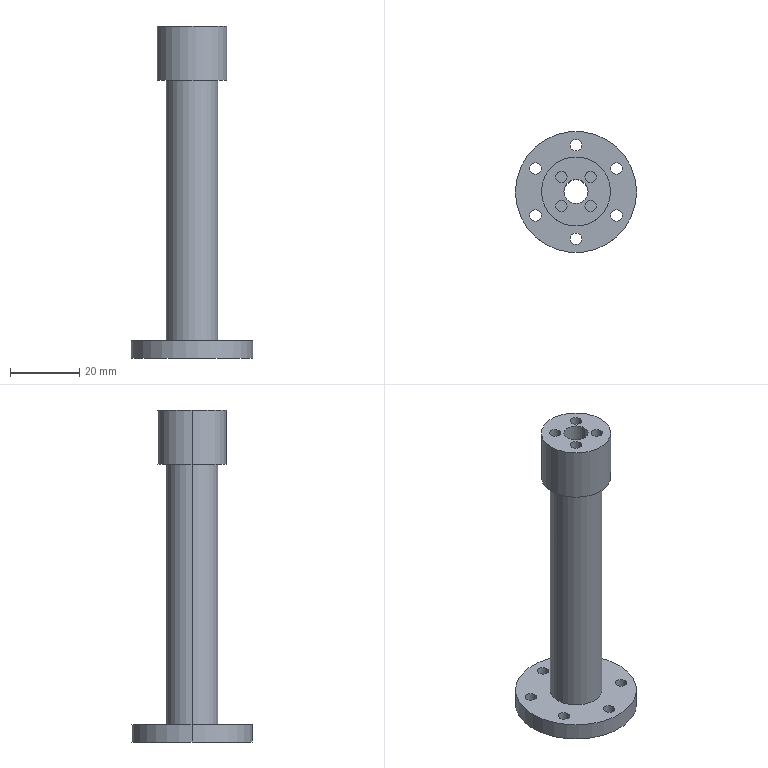Part | SolidWorks | features ICE 5, Extrusion 1 | 1 solid | 36 faces | box 35 x 35 x 95.91 mm | volume 18807 mm3 | cylinder 28 | plane 8 | commonest cylinder face diameters 3.3 x20 7 x2 15 x2 20 x2 35 x2
STEP:
#1=CARTESIAN_POINT('',(2.593,4.243,87.91));
#2=VERTEX_POINT('',#1);
#3=CARTESIAN_POINT('',(5.893,4.243,87.91));
#4=VERTEX_POINT('',#3);
#5=CARTESIAN_POINT('',(4.243,4.243,87.91));
#6=DIRECTION('',(0.,0.,1.));
#7=DIRECTION('',(1.,0.,0.));
#8=AXIS2_PLACEMENT_3D('',#5,#6,#7);
#9=CIRCLE('',#8,1.65);
#10=EDGE_CURVE('',#2,#4,#9,.T.);
#11=ORIENTED_EDGE('',*,*,#10,.F.);
#12=CARTESIAN_POINT('',(2.593,4.243,95.91));
#13=VERTEX_POINT('',#12);
#14=CARTESIAN_POINT('',(2.593,4.243,87.91));
#15=DIRECTION('',(0.,0.,1.));
#16=VECTOR('',#15,1000.);
#17=LINE('',#14,#16);
#18=EDGE_CURVE('',#2,#13,#17,.T.);
#19=ORIENTED_EDGE('',*,*,#18,.T.);
#20=CARTESIAN_POINT('',(5.893,4.243,95.91));
#21=VERTEX_POINT('',#20);
#22=CARTESIAN_POINT('',(4.243,4.243,95.91));
#23=DIRECTION('',(0.,0.,1.));
#24=DIRECTION('',(1.,0.,0.));
#25=AXIS2_PLACEMENT_3D('',#22,#23,#24);
#26=CIRCLE('',#25,1.65);
#27=EDGE_CURVE('',#13,#21,#26,.T.);
#28=ORIENTED_EDGE('',*,*,#27,.T.);
#29=CARTESIAN_POINT('',(5.893,4.243,87.91));
#30=DIRECTION('',(0.,0.,1.));
#31=VECTOR('',#30,1000.);
#32=LINE('',#29,#31);
#33=EDGE_CURVE('',#4,#21,#32,.T.);
#34=ORIENTED_EDGE('',*,*,#33,.F.);
#35=EDGE_LOOP('',(#11,#19,#28,#34));
#36=FACE_OUTER_BOUND('',#35,.T.);
#37=CARTESIAN_POINT('',(4.243,4.243,87.91));
#38=DIRECTION('',(0.,0.,1.));
#39=DIRECTION('',(1.,0.,0.));
#40=AXIS2_PLACEMENT_3D('',#37,#38,#39);
#41=CYLINDRICAL_SURFACE('',#40,1.65);
#42=ADVANCED_FACE('',(#36),#41,.F.);
#43=CARTESIAN_POINT('',(2.593,-4.243,87.91));
#44=VERTEX_POINT('',#43);
#45=CARTESIAN_POINT('',(5.893,-4.243,87.91));
#46=VERTEX_POINT('',#45);
#47=CARTESIAN_POINT('',(4.243,-4.243,87.91));
#48=DIRECTION('',(0.,0.,1.));
#49=DIRECTION('',(1.,0.,0.));
#50=AXIS2_PLACEMENT_3D('',#47,#48,#49);
#51=CIRCLE('',#50,1.65);
#52=EDGE_CURVE('',#44,#46,#51,.T.);
#53=ORIENTED_EDGE('',*,*,#52,.F.);
#54=CARTESIAN_POINT('',(2.593,-4.243,95.91));
#55=VERTEX_POINT('',#54);
#56=CARTESIAN_POINT('',(2.593,-4.243,87.91));
#57=DIRECTION('',(0.,0.,1.));
#58=VECTOR('',#57,1000.);
#59=LINE('',#56,#58);
#60=EDGE_CURVE('',#44,#55,#59,.T.);
#61=ORIENTED_EDGE('',*,*,#60,.T.);
#62=CARTESIAN_POINT('',(5.893,-4.243,95.91));
#63=VERTEX_POINT('',#62);
#64=CARTESIAN_POINT('',(4.243,-4.243,95.91));
#65=DIRECTION('',(0.,0.,1.));
#66=DIRECTION('',(1.,0.,0.));
#67=AXIS2_PLACEMENT_3D('',#64,#65,#66);
#68=CIRCLE('',#67,1.65);
#69=EDGE_CURVE('',#55,#63,#68,.T.);
#70=ORIENTED_EDGE('',*,*,#69,.T.);
#71=CARTESIAN_POINT('',(5.893,-4.243,87.91));
#72=DIRECTION('',(0.,0.,1.));
#73=VECTOR('',#72,1000.);
#74=LINE('',#71,#73);
#75=EDGE_CURVE('',#46,#63,#74,.T.);
#76=ORIENTED_EDGE('',*,*,#75,.F.);
#77=EDGE_LOOP('',(#53,#61,#70,#76));
#78=FACE_OUTER_BOUND('',#77,.T.);
#79=CARTESIAN_POINT('',(4.243,-4.243,87.91));
#80=DIRECTION('',(0.,0.,1.));
#81=DIRECTION('',(1.,0.,0.));
#82=AXIS2_PLACEMENT_3D('',#79,#80,#81);
#83=CYLINDRICAL_SURFACE('',#82,1.65);
#84=ADVANCED_FACE('',(#78),#83,.F.);
#85=CARTESIAN_POINT('',(-5.893,-4.243,87.91));
#86=VERTEX_POINT('',#85);
#87=CARTESIAN_POINT('',(-2.593,-4.243,87.91));
#88=VERTEX_POINT('',#87);
#89=CARTESIAN_POINT('',(-4.243,-4.243,87.91));
#90=DIRECTION('',(0.,0.,1.));
#91=DIRECTION('',(1.,0.,0.));
#92=AXIS2_PLACEMENT_3D('',#89,#90,#91);
#93=CIRCLE('',#92,1.65);
#94=EDGE_CURVE('',#86,#88,#93,.T.);
#95=ORIENTED_EDGE('',*,*,#94,.F.);
#96=CARTESIAN_POINT('',(-5.893,-4.243,95.91));
#97=VERTEX_POINT('',#96);
#98=CARTESIAN_POINT('',(-5.893,-4.243,87.91));
#99=DIRECTION('',(0.,0.,1.));
#100=VECTOR('',#99,1000.);
#101=LINE('',#98,#100);
#102=EDGE_CURVE('',#86,#97,#101,.T.);
#103=ORIENTED_EDGE('',*,*,#102,.T.);
#104=CARTESIAN_POINT('',(-2.593,-4.243,95.91));
#105=VERTEX_POINT('',#104);
#106=CARTESIAN_POINT('',(-4.243,-4.243,95.91));
#107=DIRECTION('',(0.,0.,1.));
#108=DIRECTION('',(1.,0.,0.));
#109=AXIS2_PLACEMENT_3D('',#106,#107,#108);
#110=CIRCLE('',#109,1.65);
#111=EDGE_CURVE('',#97,#105,#110,.T.);
#112=ORIENTED_EDGE('',*,*,#111,.T.);
#113=CARTESIAN_POINT('',(-2.593,-4.243,87.91));
#114=DIRECTION('',(0.,0.,1.));
#115=VECTOR('',#114,1000.);
#116=LINE('',#113,#115);
#117=EDGE_CURVE('',#88,#105,#116,.T.);
#118=ORIENTED_EDGE('',*,*,#117,.F.);
#119=EDGE_LOOP('',(#95,#103,#112,#118));
#120=FACE_OUTER_BOUND('',#119,.T.);
#121=CARTESIAN_POINT('',(-4.243,-4.243,87.91));
#122=DIRECTION('',(0.,0.,1.));
#123=DIRECTION('',(1.,0.,0.));
#124=AXIS2_PLACEMENT_3D('',#121,#122,#123);
#125=CYLINDRICAL_SURFACE('',#124,1.65);
#126=ADVANCED_FACE('',(#120),#125,.F.);
#127=CARTESIAN_POINT('',(-5.893,4.243,87.91));
#128=VERTEX_POINT('',#127);
#129=CARTESIAN_POINT('',(-2.593,4.243,87.91));
#130=VERTEX_POINT('',#129);
#131=CARTESIAN_POINT('',(-4.243,4.243,87.91));
#132=DIRECTION('',(0.,0.,1.));
#133=DIRECTION('',(1.,0.,0.));
#134=AXIS2_PLACEMENT_3D('',#131,#132,#133);
#135=CIRCLE('',#134,1.65);
#136=EDGE_CURVE('',#128,#130,#135,.T.);
#137=ORIENTED_EDGE('',*,*,#136,.F.);
#138=CARTESIAN_POINT('',(-5.893,4.243,95.91));
#139=VERTEX_POINT('',#138);
#140=CARTESIAN_POINT('',(-5.893,4.243,87.91));
#141=DIRECTION('',(0.,0.,1.));
#142=VECTOR('',#141,1000.);
#143=LINE('',#140,#142);
#144=EDGE_CURVE('',#128,#139,#143,.T.);
#145=ORIENTED_EDGE('',*,*,#144,.T.);
#146=CARTESIAN_POINT('',(-2.593,4.243,95.91));
#147=VERTEX_POINT('',#146);
#148=CARTESIAN_POINT('',(-4.243,4.243,95.91));
#149=DIRECTION('',(0.,0.,1.));
#150=DIRECTION('',(1.,0.,0.));
#151=AXIS2_PLACEMENT_3D('',#148,#149,#150);
#152=CIRCLE('',#151,1.65);
#153=EDGE_CURVE('',#139,#147,#152,.T.);
#154=ORIENTED_EDGE('',*,*,#153,.T.);
#155=CARTESIAN_POINT('',(-2.593,4.243,87.91));
#156=DIRECTION('',(0.,0.,1.));
#157=VECTOR('',#156,1000.);
#158=LINE('',#155,#157);
#159=EDGE_CURVE('',#130,#147,#158,.T.);
#160=ORIENTED_EDGE('',*,*,#159,.F.);
#161=EDGE_LOOP('',(#137,#145,#154,#160));
#162=FACE_OUTER_BOUND('',#161,.T.);
#163=CARTESIAN_POINT('',(-4.243,4.243,87.91));
#164=DIRECTION('',(0.,0.,1.));
#165=DIRECTION('',(1.,0.,0.));
#166=AXIS2_PLACEMENT_3D('',#163,#164,#165);
#167=CYLINDRICAL_SURFACE('',#166,1.65);
#168=ADVANCED_FACE('',(#162),#167,.F.);
#169=CARTESIAN_POINT('',(10.,0.,80.25));
#170=VERTEX_POINT('',#169);
#171=CARTESIAN_POINT('',(-10.,0.,80.25));
#172=VERTEX_POINT('',#171);
#173=CARTESIAN_POINT('',(0.,0.,80.25));
#174=DIRECTION('',(0.,0.,1.));
#175=DIRECTION('',(1.,0.,0.));
#176=AXIS2_PLACEMENT_3D('',#173,#174,#175);
#177=CIRCLE('',#176,10.);
#178=EDGE_CURVE('',#170,#172,#177,.T.);
#179=ORIENTED_EDGE('',*,*,#178,.T.);
#180=CARTESIAN_POINT('',(-10.,0.,95.91));
#181=VERTEX_POINT('',#180);
#182=CARTESIAN_POINT('',(-10.,0.,80.25));
#183=DIRECTION('',(0.,0.,1.));
#184=VECTOR('',#183,1000.);
#185=LINE('',#182,#184);
#186=EDGE_CURVE('',#172,#181,#185,.T.);
#187=ORIENTED_EDGE('',*,*,#186,.T.);
#188=CARTESIAN_POINT('',(10.,0.,95.91));
#189=VERTEX_POINT('',#188);
#190=CARTESIAN_POINT('',(0.,0.,95.91));
#191=DIRECTION('',(0.,0.,1.));
#192=DIRECTION('',(1.,0.,0.));
#193=AXIS2_PLACEMENT_3D('',#190,#191,#192);
#194=CIRCLE('',#193,10.);
#195=EDGE_CURVE('',#189,#181,#194,.T.);
#196=ORIENTED_EDGE('',*,*,#195,.F.);
#197=CARTESIAN_POINT('',(10.,0.,80.25));
#198=DIRECTION('',(0.,0.,1.));
#199=VECTOR('',#198,1000.);
#200=LINE('',#197,#199);
#201=EDGE_CURVE('',#170,#189,#200,.T.);
#202=ORIENTED_EDGE('',*,*,#201,.F.);
#203=EDGE_LOOP('',(#179,#187,#196,#202));
#204=FACE_OUTER_BOUND('',#203,.T.);
#205=CARTESIAN_POINT('',(0.,0.,80.25));
#206=DIRECTION('',(0.,0.,1.));
#207=DIRECTION('',(1.,0.,0.));
#208=AXIS2_PLACEMENT_3D('',#205,#206,#207);
#209=CYLINDRICAL_SURFACE('',#208,10.);
#210=ADVANCED_FACE('',(#204),#209,.T.);
#211=CARTESIAN_POINT('',(-1.65,13.5,5.));
#212=VERTEX_POINT('',#211);
#213=CARTESIAN_POINT('',(1.65,13.5,5.));
#214=VERTEX_POINT('',#213);
#215=CARTESIAN_POINT('',(0.,13.5,5.));
#216=DIRECTION('',(0.,0.,1.));
#217=DIRECTION('',(1.,0.,0.));
#218=AXIS2_PLACEMENT_3D('',#215,#216,#217);
#219=CIRCLE('',#218,1.65);
#220=EDGE_CURVE('',#212,#214,#219,.T.);
#221=ORIENTED_EDGE('',*,*,#220,.T.);
#222=CARTESIAN_POINT('',(1.65,13.5,0.));
#223=VERTEX_POINT('',#222);
#224=CARTESIAN_POINT('',(1.65,13.5,1000.));
#225=DIRECTION('',(0.,0.,-1.));
#226=VECTOR('',#225,1000.);
#227=LINE('',#224,#226);
#228=EDGE_CURVE('',#214,#223,#227,.T.);
#229=ORIENTED_EDGE('',*,*,#228,.T.);
#230=CARTESIAN_POINT('',(-1.65,13.5,0.));
#231=VERTEX_POINT('',#230);
#232=CARTESIAN_POINT('',(0.,13.5,0.));
#233=DIRECTION('',(0.,0.,-1.));
#234=DIRECTION('',(-1.,0.,0.));
#235=AXIS2_PLACEMENT_3D('',#232,#233,#234);
#236=CIRCLE('',#235,1.65);
#237=EDGE_CURVE('',#223,#231,#236,.T.);
#238=ORIENTED_EDGE('',*,*,#237,.T.);
#239=CARTESIAN_POINT('',(-1.65,13.5,1000.));
#240=DIRECTION('',(0.,0.,-1.));
#241=VECTOR('',#240,1000.);
#242=LINE('',#239,#241);
#243=EDGE_CURVE('',#212,#231,#242,.T.);
#244=ORIENTED_EDGE('',*,*,#243,.F.);
#245=EDGE_LOOP('',(#221,#229,#238,#244));
#246=FACE_OUTER_BOUND('',#245,.T.);
#247=CARTESIAN_POINT('',(0.,13.5,1000.));
#248=DIRECTION('',(0.,0.,-1.));
#249=DIRECTION('',(-1.,0.,0.));
#250=AXIS2_PLACEMENT_3D('',#247,#248,#249);
#251=CYLINDRICAL_SURFACE('',#250,1.65);
#252=ADVANCED_FACE('',(#246),#251,.F.);
#253=CARTESIAN_POINT('',(-13.341,6.75,5.));
#254=VERTEX_POINT('',#253);
#255=CARTESIAN_POINT('',(-10.041,6.75,5.));
#256=VERTEX_POINT('',#255);
#257=CARTESIAN_POINT('',(-11.691,6.75,5.));
#258=DIRECTION('',(0.,0.,1.));
#259=DIRECTION('',(1.,0.,0.));
#260=AXIS2_PLACEMENT_3D('',#257,#258,#259);
#261=CIRCLE('',#260,1.65);
#262=EDGE_CURVE('',#254,#256,#261,.T.);
#263=ORIENTED_EDGE('',*,*,#262,.T.);
#264=CARTESIAN_POINT('',(-10.041,6.75,0.));
#265=VERTEX_POINT('',#264);
#266=CARTESIAN_POINT('',(-10.041,6.75,1000.));
#267=DIRECTION('',(0.,0.,-1.));
#268=VECTOR('',#267,1000.);
#269=LINE('',#266,#268);
#270=EDGE_CURVE('',#256,#265,#269,.T.);
#271=ORIENTED_EDGE('',*,*,#270,.T.);
#272=CARTESIAN_POINT('',(-13.341,6.75,0.));
#273=VERTEX_POINT('',#272);
#274=CARTESIAN_POINT('',(-11.691,6.75,0.));
#275=DIRECTION('',(0.,0.,-1.));
#276=DIRECTION('',(-1.,0.,0.));
#277=AXIS2_PLACEMENT_3D('',#274,#275,#276);
#278=CIRCLE('',#277,1.65);
#279=EDGE_CURVE('',#265,#273,#278,.T.);
#280=ORIENTED_EDGE('',*,*,#279,.T.);
#281=CARTESIAN_POINT('',(-13.341,6.75,1000.));
#282=DIRECTION('',(0.,0.,-1.));
#283=VECTOR('',#282,1000.);
#284=LINE('',#281,#283);
#285=EDGE_CURVE('',#254,#273,#284,.T.);
#286=ORIENTED_EDGE('',*,*,#285,.F.);
#287=EDGE_LOOP('',(#263,#271,#280,#286));
#288=FACE_OUTER_BOUND('',#287,.T.);
#289=CARTESIAN_POINT('',(-11.691,6.75,1000.));
#290=DIRECTION('',(0.,0.,-1.));
#291=DIRECTION('',(-1.,0.,0.));
#292=AXIS2_PLACEMENT_3D('',#289,#290,#291);
#293=CYLINDRICAL_SURFACE('',#292,1.65);
#294=ADVANCED_FACE('',(#288),#293,.F.);
#295=CARTESIAN_POINT('',(-13.341,-6.75,5.));
#296=VERTEX_POINT('',#295);
#297=CARTESIAN_POINT('',(-10.041,-6.75,5.));
#298=VERTEX_POINT('',#297);
#299=CARTESIAN_POINT('',(-11.691,-6.75,5.));
#300=DIRECTION('',(0.,0.,1.));
#301=DIRECTION('',(1.,0.,0.));
#302=AXIS2_PLACEMENT_3D('',#299,#300,#301);
#303=CIRCLE('',#302,1.65);
#304=EDGE_CURVE('',#296,#298,#303,.T.);
#305=ORIENTED_EDGE('',*,*,#304,.T.);
#306=CARTESIAN_POINT('',(-10.041,-6.75,0.));
#307=VERTEX_POINT('',#306);
#308=CARTESIAN_POINT('',(-10.041,-6.75,1000.));
#309=DIRECTION('',(0.,0.,-1.));
#310=VECTOR('',#309,1000.);
#311=LINE('',#308,#310);
#312=EDGE_CURVE('',#298,#307,#311,.T.);
#313=ORIENTED_EDGE('',*,*,#312,.T.);
#314=CARTESIAN_POINT('',(-13.341,-6.75,0.));
#315=VERTEX_POINT('',#314);
#316=CARTESIAN_POINT('',(-11.691,-6.75,0.));
#317=DIRECTION('',(0.,0.,-1.));
#318=DIRECTION('',(-1.,0.,0.));
#319=AXIS2_PLACEMENT_3D('',#316,#317,#318);
#320=CIRCLE('',#319,1.65);
#321=EDGE_CURVE('',#307,#315,#320,.T.);
#322=ORIENTED_EDGE('',*,*,#321,.T.);
#323=CARTESIAN_POINT('',(-13.341,-6.75,1000.));
#324=DIRECTION('',(0.,0.,-1.));
#325=VECTOR('',#324,1000.);
#326=LINE('',#323,#325);
#327=EDGE_CURVE('',#296,#315,#326,.T.);
#328=ORIENTED_EDGE('',*,*,#327,.F.);
#329=EDGE_LOOP('',(#305,#313,#322,#328));
#330=FACE_OUTER_BOUND('',#329,.T.);
#331=CARTESIAN_POINT('',(-11.691,-6.75,1000.));
#332=DIRECTION('',(0.,0.,-1.));
#333=DIRECTION('',(-1.,0.,0.));
#334=AXIS2_PLACEMENT_3D('',#331,#332,#333);
#335=CYLINDRICAL_SURFACE('',#334,1.65);
#336=ADVANCED_FACE('',(#330),#335,.F.);
#337=CARTESIAN_POINT('',(-1.65,-13.5,5.));
#338=VERTEX_POINT('',#337);
#339=CARTESIAN_POINT('',(1.65,-13.5,5.));
#340=VERTEX_POINT('',#339);
#341=CARTESIAN_POINT('',(0.,-13.5,5.));
#342=DIRECTION('',(0.,0.,1.));
#343=DIRECTION('',(1.,0.,0.));
#344=AXIS2_PLACEMENT_3D('',#341,#342,#343);
#345=CIRCLE('',#344,1.65);
#346=EDGE_CURVE('',#338,#340,#345,.T.);
#347=ORIENTED_EDGE('',*,*,#346,.T.);
#348=CARTESIAN_POINT('',(1.65,-13.5,0.));
#349=VERTEX_POINT('',#348);
#350=CARTESIAN_POINT('',(1.65,-13.5,1000.));
#351=DIRECTION('',(0.,0.,-1.));
#352=VECTOR('',#351,1000.);
#353=LINE('',#350,#352);
#354=EDGE_CURVE('',#340,#349,#353,.T.);
#355=ORIENTED_EDGE('',*,*,#354,.T.);
#356=CARTESIAN_POINT('',(-1.65,-13.5,0.));
#357=VERTEX_POINT('',#356);
#358=CARTESIAN_POINT('',(0.,-13.5,0.));
#359=DIRECTION('',(0.,0.,-1.));
#360=DIRECTION('',(-1.,0.,0.));
#361=AXIS2_PLACEMENT_3D('',#358,#359,#360);
#362=CIRCLE('',#361,1.65);
#363=EDGE_CURVE('',#349,#357,#362,.T.);
#364=ORIENTED_EDGE('',*,*,#363,.T.);
#365=CARTESIAN_POINT('',(-1.65,-13.5,1000.));
#366=DIRECTION('',(0.,0.,-1.));
#367=VECTOR('',#366,1000.);
#368=LINE('',#365,#367);
#369=EDGE_CURVE('',#338,#357,#368,.T.);
#370=ORIENTED_EDGE('',*,*,#369,.F.);
#371=EDGE_LOOP('',(#347,#355,#364,#370));
#372=FACE_OUTER_BOUND('',#371,.T.);
#373=CARTESIAN_POINT('',(0.,-13.5,1000.));
#374=DIRECTION('',(0.,0.,-1.));
#375=DIRECTION('',(-1.,0.,0.));
#376=AXIS2_PLACEMENT_3D('',#373,#374,#375);
#377=CYLINDRICAL_SURFACE('',#376,1.65);
#378=ADVANCED_FACE('',(#372),#377,.F.);
#379=CARTESIAN_POINT('',(10.041,-6.75,5.));
#380=VERTEX_POINT('',#379);
#381=CARTESIAN_POINT('',(13.341,-6.75,5.));
#382=VERTEX_POINT('',#381);
#383=CARTESIAN_POINT('',(11.691,-6.75,5.));
#384=DIRECTION('',(0.,0.,1.));
#385=DIRECTION('',(1.,0.,0.));
#386=AXIS2_PLACEMENT_3D('',#383,#384,#385);
#387=CIRCLE('',#386,1.65);
#388=EDGE_CURVE('',#380,#382,#387,.T.);
#389=ORIENTED_EDGE('',*,*,#388,.T.);
#390=CARTESIAN_POINT('',(13.341,-6.75,0.));
#391=VERTEX_POINT('',#390);
#392=CARTESIAN_POINT('',(13.341,-6.75,1000.));
#393=DIRECTION('',(0.,0.,-1.));
#394=VECTOR('',#393,1000.);
#395=LINE('',#392,#394);
#396=EDGE_CURVE('',#382,#391,#395,.T.);
#397=ORIENTED_EDGE('',*,*,#396,.T.);
#398=CARTESIAN_POINT('',(10.041,-6.75,0.));
#399=VERTEX_POINT('',#398);
#400=CARTESIAN_POINT('',(11.691,-6.75,0.));
#401=DIRECTION('',(0.,0.,-1.));
#402=DIRECTION('',(-1.,0.,0.));
#403=AXIS2_PLACEMENT_3D('',#400,#401,#402);
#404=CIRCLE('',#403,1.65);
#405=EDGE_CURVE('',#391,#399,#404,.T.);
#406=ORIENTED_EDGE('',*,*,#405,.T.);
#407=CARTESIAN_POINT('',(10.041,-6.75,1000.));
#408=DIRECTION('',(0.,0.,-1.));
#409=VECTOR('',#408,1000.);
#410=LINE('',#407,#409);
#411=EDGE_CURVE('',#380,#399,#410,.T.);
#412=ORIENTED_EDGE('',*,*,#411,.F.);
#413=EDGE_LOOP('',(#389,#397,#406,#412));
#414=FACE_OUTER_BOUND('',#413,.T.);
#415=CARTESIAN_POINT('',(11.691,-6.75,1000.));
#416=DIRECTION('',(0.,0.,-1.));
#417=DIRECTION('',(-1.,0.,0.));
#418=AXIS2_PLACEMENT_3D('',#415,#416,#417);
#419=CYLINDRICAL_SURFACE('',#418,1.65);
#420=ADVANCED_FACE('',(#414),#419,.F.);
#421=CARTESIAN_POINT('',(10.041,6.75,5.));
#422=VERTEX_POINT('',#421);
#423=CARTESIAN_POINT('',(13.341,6.75,5.));
#424=VERTEX_POINT('',#423);
#425=CARTESIAN_POINT('',(11.691,6.75,5.));
#426=DIRECTION('',(0.,0.,1.));
#427=DIRECTION('',(1.,0.,0.));
#428=AXIS2_PLACEMENT_3D('',#425,#426,#427);
#429=CIRCLE('',#428,1.65);
#430=EDGE_CURVE('',#422,#424,#429,.T.);
#431=ORIENTED_EDGE('',*,*,#430,.T.);
#432=CARTESIAN_POINT('',(13.341,6.75,0.));
#433=VERTEX_POINT('',#432);
#434=CARTESIAN_POINT('',(13.341,6.75,1000.));
#435=DIRECTION('',(0.,0.,-1.));
#436=VECTOR('',#435,1000.);
#437=LINE('',#434,#436);
#438=EDGE_CURVE('',#424,#433,#437,.T.);
#439=ORIENTED_EDGE('',*,*,#438,.T.);
#440=CARTESIAN_POINT('',(10.041,6.75,0.));
#441=VERTEX_POINT('',#440);
#442=CARTESIAN_POINT('',(11.691,6.75,0.));
#443=DIRECTION('',(0.,0.,-1.));
#444=DIRECTION('',(-1.,0.,0.));
#445=AXIS2_PLACEMENT_3D('',#442,#443,#444);
#446=CIRCLE('',#445,1.65);
#447=EDGE_CURVE('',#433,#441,#446,.T.);
#448=ORIENTED_EDGE('',*,*,#447,.T.);
#449=CARTESIAN_POINT('',(10.041,6.75,1000.));
#450=DIRECTION('',(0.,0.,-1.));
#451=VECTOR('',#450,1000.);
#452=LINE('',#449,#451);
#453=EDGE_CURVE('',#422,#441,#452,.T.);
#454=ORIENTED_EDGE('',*,*,#453,.F.);
#455=EDGE_LOOP('',(#431,#439,#448,#454));
#456=FACE_OUTER_BOUND('',#455,.T.);
#457=CARTESIAN_POINT('',(11.691,6.75,1000.));
#458=DIRECTION('',(0.,0.,-1.));
#459=DIRECTION('',(-1.,0.,0.));
#460=AXIS2_PLACEMENT_3D('',#457,#458,#459);
#461=CYLINDRICAL_SURFACE('',#460,1.65);
#462=ADVANCED_FACE('',(#456),#461,.F.);
#463=CARTESIAN_POINT('',(-3.5,0.,95.91));
#464=VERTEX_POINT('',#463);
#465=CARTESIAN_POINT('',(3.5,0.,95.91));
#466=VERTEX_POINT('',#465);
#467=CARTESIAN_POINT('',(0.,0.,95.91));
#468=DIRECTION('',(0.,0.,1.));
#469=DIRECTION('',(1.,0.,0.));
#470=AXIS2_PLACEMENT_3D('',#467,#468,#469);
#471=CIRCLE('',#470,3.5);
#472=EDGE_CURVE('',#464,#466,#471,.T.);
#473=ORIENTED_EDGE('',*,*,#472,.T.);
#474=CARTESIAN_POINT('',(3.5,0.,0.));
#475=VERTEX_POINT('',#474);
#476=CARTESIAN_POINT('',(3.5,0.,1000.));
#477=DIRECTION('',(0.,0.,-1.));
#478=VECTOR('',#477,1000.);
#479=LINE('',#476,#478);
#480=EDGE_CURVE('',#466,#475,#479,.T.);
#481=ORIENTED_EDGE('',*,*,#480,.T.);
#482=CARTESIAN_POINT('',(-3.5,0.,0.));
#483=VERTEX_POINT('',#482);
#484=CARTESIAN_POINT('',(0.,0.,0.));
#485=DIRECTION('',(0.,0.,-1.));
#486=DIRECTION('',(-1.,0.,0.));
#487=AXIS2_PLACEMENT_3D('',#484,#485,#486);
#488=CIRCLE('',#487,3.5);
#489=EDGE_CURVE('',#475,#483,#488,.T.);
#490=ORIENTED_EDGE('',*,*,#489,.T.);
#491=CARTESIAN_POINT('',(-3.5,0.,1000.));
#492=DIRECTION('',(0.,0.,-1.));
#493=VECTOR('',#492,1000.);
#494=LINE('',#491,#493);
#495=EDGE_CURVE('',#464,#483,#494,.T.);
#496=ORIENTED_EDGE('',*,*,#495,.F.);
#497=EDGE_LOOP('',(#473,#481,#490,#496));
#498=FACE_OUTER_BOUND('',#497,.T.);
#499=CARTESIAN_POINT('',(0.,0.,1000.));
#500=DIRECTION('',(0.,0.,-1.));
#501=DIRECTION('',(-1.,0.,0.));
#502=AXIS2_PLACEMENT_3D('',#499,#500,#501);
#503=CYLINDRICAL_SURFACE('',#502,3.5);
#504=ADVANCED_FACE('',(#498),#503,.F.);
#505=CARTESIAN_POINT('',(17.5,0.,5.));
#506=VERTEX_POINT('',#505);
#507=CARTESIAN_POINT('',(-17.5,0.,5.));
#508=VERTEX_POINT('',#507);
#509=CARTESIAN_POINT('',(0.,0.,5.));
#510=DIRECTION('',(0.,0.,1.));
#511=DIRECTION('',(1.,0.,0.));
#512=AXIS2_PLACEMENT_3D('',#509,#510,#511);
#513=CIRCLE('',#512,17.5);
#514=EDGE_CURVE('',#506,#508,#513,.T.);
#515=ORIENTED_EDGE('',*,*,#514,.F.);
#516=CARTESIAN_POINT('',(17.5,0.,0.));
#517=VERTEX_POINT('',#516);
#518=CARTESIAN_POINT('',(17.5,0.,5.));
#519=DIRECTION('',(0.,0.,-1.));
#520=VECTOR('',#519,1000.);
#521=LINE('',#518,#520);
#522=EDGE_CURVE('',#506,#517,#521,.T.);
#523=ORIENTED_EDGE('',*,*,#522,.T.);
#524=CARTESIAN_POINT('',(-17.5,0.,0.));
#525=VERTEX_POINT('',#524);
#526=CARTESIAN_POINT('',(0.,0.,0.));
#527=DIRECTION('',(0.,0.,1.));
#528=DIRECTION('',(1.,0.,0.));
#529=AXIS2_PLACEMENT_3D('',#526,#527,#528);
#530=CIRCLE('',#529,17.5);
#531=EDGE_CURVE('',#517,#525,#530,.T.);
#532=ORIENTED_EDGE('',*,*,#531,.T.);
#533=CARTESIAN_POINT('',(-17.5,0.,5.));
#534=DIRECTION('',(0.,0.,-1.));
#535=VECTOR('',#534,1000.);
#536=LINE('',#533,#535);
#537=EDGE_CURVE('',#508,#525,#536,.T.);
#538=ORIENTED_EDGE('',*,*,#537,.F.);
#539=EDGE_LOOP('',(#515,#523,#532,#538));
#540=FACE_OUTER_BOUND('',#539,.T.);
#541=CARTESIAN_POINT('',(0.,0.,5.));
#542=DIRECTION('',(0.,0.,-1.));
#543=DIRECTION('',(-1.,0.,0.));
#544=AXIS2_PLACEMENT_3D('',#541,#542,#543);
#545=CYLINDRICAL_SURFACE('',#544,17.5);
#546=ADVANCED_FACE('',(#540),#545,.T.);
#547=CARTESIAN_POINT('',(7.5,0.,80.25));
#548=VERTEX_POINT('',#547);
#549=CARTESIAN_POINT('',(-7.5,0.,80.25));
#550=VERTEX_POINT('',#549);
#551=CARTESIAN_POINT('',(0.,0.,80.25));
#552=DIRECTION('',(0.,0.,1.));
#553=DIRECTION('',(1.,0.,0.));
#554=AXIS2_PLACEMENT_3D('',#551,#552,#553);
#555=CIRCLE('',#554,7.5);
#556=EDGE_CURVE('',#548,#550,#555,.T.);
#557=ORIENTED_EDGE('',*,*,#556,.F.);
#558=CARTESIAN_POINT('',(7.5,0.,5.));
#559=VERTEX_POINT('',#558);
#560=CARTESIAN_POINT('',(7.5,0.,95.91));
#561=DIRECTION('',(0.,0.,-1.));
#562=VECTOR('',#561,1000.);
#563=LINE('',#560,#562);
#564=EDGE_CURVE('',#548,#559,#563,.T.);
#565=ORIENTED_EDGE('',*,*,#564,.T.);
#566=CARTESIAN_POINT('',(-7.5,0.,5.));
#567=VERTEX_POINT('',#566);
#568=CARTESIAN_POINT('',(0.,0.,5.));
#569=DIRECTION('',(0.,0.,1.));
#570=DIRECTION('',(1.,0.,0.));
#571=AXIS2_PLACEMENT_3D('',#568,#569,#570);
#572=CIRCLE('',#571,7.5);
#573=EDGE_CURVE('',#559,#567,#572,.T.);
#574=ORIENTED_EDGE('',*,*,#573,.T.);
#575=CARTESIAN_POINT('',(-7.5,0.,95.91));
#576=DIRECTION('',(0.,0.,-1.));
#577=VECTOR('',#576,1000.);
#578=LINE('',#575,#577);
#579=EDGE_CURVE('',#550,#567,#578,.T.);
#580=ORIENTED_EDGE('',*,*,#579,.F.);
#581=EDGE_LOOP('',(#557,#565,#574,#580));
#582=FACE_OUTER_BOUND('',#581,.T.);
#583=CARTESIAN_POINT('',(0.,0.,95.91));
#584=DIRECTION('',(0.,0.,-1.));
#585=DIRECTION('',(-1.,0.,0.));
#586=AXIS2_PLACEMENT_3D('',#583,#584,#585);
#587=CYLINDRICAL_SURFACE('',#586,7.5);
#588=ADVANCED_FACE('',(#582),#587,.T.);
#589=ORIENTED_EDGE('',*,*,#564,.F.);
#590=CARTESIAN_POINT('',(0.,0.,80.25));
#591=DIRECTION('',(0.,0.,1.));
#592=DIRECTION('',(1.,0.,0.));
#593=AXIS2_PLACEMENT_3D('',#590,#591,#592);
#594=CIRCLE('',#593,7.5);
#595=EDGE_CURVE('',#550,#548,#594,.T.);
#596=ORIENTED_EDGE('',*,*,#595,.F.);
#597=ORIENTED_EDGE('',*,*,#579,.T.);
#598=CARTESIAN_POINT('',(0.,0.,5.));
#599=DIRECTION('',(0.,0.,1.));
#600=DIRECTION('',(1.,0.,0.));
#601=AXIS2_PLACEMENT_3D('',#598,#599,#600);
#602=CIRCLE('',#601,7.5);
#603=EDGE_CURVE('',#567,#559,#602,.T.);
#604=ORIENTED_EDGE('',*,*,#603,.T.);
#605=EDGE_LOOP('',(#589,#596,#597,#604));
#606=FACE_OUTER_BOUND('',#605,.T.);
#607=CARTESIAN_POINT('',(0.,0.,95.91));
#608=DIRECTION('',(0.,0.,-1.));
#609=DIRECTION('',(-1.,0.,0.));
#610=AXIS2_PLACEMENT_3D('',#607,#608,#609);
#611=CYLINDRICAL_SURFACE('',#610,7.5);
#612=ADVANCED_FACE('',(#606),#611,.T.);
#613=ORIENTED_EDGE('',*,*,#522,.F.);
#614=CARTESIAN_POINT('',(0.,0.,5.));
#615=DIRECTION('',(0.,0.,1.));
#616=DIRECTION('',(1.,0.,0.));
#617=AXIS2_PLACEMENT_3D('',#614,#615,#616);
#618=CIRCLE('',#617,17.5);
#619=EDGE_CURVE('',#508,#506,#618,.T.);
#620=ORIENTED_EDGE('',*,*,#619,.F.);
#621=ORIENTED_EDGE('',*,*,#537,.T.);
#622=CARTESIAN_POINT('',(0.,0.,0.));
#623=DIRECTION('',(0.,0.,1.));
#624=DIRECTION('',(1.,0.,0.));
#625=AXIS2_PLACEMENT_3D('',#622,#623,#624);
#626=CIRCLE('',#625,17.5);
#627=EDGE_CURVE('',#525,#517,#626,.T.);
#628=ORIENTED_EDGE('',*,*,#627,.T.);
#629=EDGE_LOOP('',(#613,#620,#621,#628));
#630=FACE_OUTER_BOUND('',#629,.T.);
#631=CARTESIAN_POINT('',(0.,0.,5.));
#632=DIRECTION('',(0.,0.,-1.));
#633=DIRECTION('',(-1.,0.,0.));
#634=AXIS2_PLACEMENT_3D('',#631,#632,#633);
#635=CYLINDRICAL_SURFACE('',#634,17.5);
#636=ADVANCED_FACE('',(#630),#635,.T.);
#637=ORIENTED_EDGE('',*,*,#220,.F.);
#638=CARTESIAN_POINT('',(0.,13.5,5.));
#639=DIRECTION('',(0.,0.,1.));
#640=DIRECTION('',(1.,0.,0.));
#641=AXIS2_PLACEMENT_3D('',#638,#639,#640);
#642=CIRCLE('',#641,1.65);
#643=EDGE_CURVE('',#214,#212,#642,.T.);
#644=ORIENTED_EDGE('',*,*,#643,.F.);
#645=EDGE_LOOP('',(#637,#644));
#646=FACE_BOUND('',#645,.T.);
#647=ORIENTED_EDGE('',*,*,#262,.F.);
#648=CARTESIAN_POINT('',(-11.691,6.75,5.));
#649=DIRECTION('',(0.,0.,1.));
#650=DIRECTION('',(1.,0.,0.));
#651=AXIS2_PLACEMENT_3D('',#648,#649,#650);
#652=CIRCLE('',#651,1.65);
#653=EDGE_CURVE('',#256,#254,#652,.T.);
#654=ORIENTED_EDGE('',*,*,#653,.F.);
#655=EDGE_LOOP('',(#647,#654));
#656=FACE_BOUND('',#655,.T.);
#657=ORIENTED_EDGE('',*,*,#304,.F.);
#658=CARTESIAN_POINT('',(-11.691,-6.75,5.));
#659=DIRECTION('',(0.,0.,1.));
#660=DIRECTION('',(1.,0.,0.));
#661=AXIS2_PLACEMENT_3D('',#658,#659,#660);
#662=CIRCLE('',#661,1.65);
#663=EDGE_CURVE('',#298,#296,#662,.T.);
#664=ORIENTED_EDGE('',*,*,#663,.F.);
#665=EDGE_LOOP('',(#657,#664));
#666=FACE_BOUND('',#665,.T.);
#667=ORIENTED_EDGE('',*,*,#346,.F.);
#668=CARTESIAN_POINT('',(0.,-13.5,5.));
#669=DIRECTION('',(0.,0.,1.));
#670=DIRECTION('',(1.,0.,0.));
#671=AXIS2_PLACEMENT_3D('',#668,#669,#670);
#672=CIRCLE('',#671,1.65);
#673=EDGE_CURVE('',#340,#338,#672,.T.);
#674=ORIENTED_EDGE('',*,*,#673,.F.);
#675=EDGE_LOOP('',(#667,#674));
#676=FACE_BOUND('',#675,.T.);
#677=ORIENTED_EDGE('',*,*,#388,.F.);
#678=CARTESIAN_POINT('',(11.691,-6.75,5.));
#679=DIRECTION('',(0.,0.,1.));
#680=DIRECTION('',(1.,0.,0.));
#681=AXIS2_PLACEMENT_3D('',#678,#679,#680);
#682=CIRCLE('',#681,1.65);
#683=EDGE_CURVE('',#382,#380,#682,.T.);
#684=ORIENTED_EDGE('',*,*,#683,.F.);
#685=EDGE_LOOP('',(#677,#684));
#686=FACE_BOUND('',#685,.T.);
#687=ORIENTED_EDGE('',*,*,#430,.F.);
#688=CARTESIAN_POINT('',(11.691,6.75,5.));
#689=DIRECTION('',(0.,0.,1.));
#690=DIRECTION('',(1.,0.,0.));
#691=AXIS2_PLACEMENT_3D('',#688,#689,#690);
#692=CIRCLE('',#691,1.65);
#693=EDGE_CURVE('',#424,#422,#692,.T.);
#694=ORIENTED_EDGE('',*,*,#693,.F.);
#695=EDGE_LOOP('',(#687,#694));
#696=FACE_BOUND('',#695,.T.);
#697=ORIENTED_EDGE('',*,*,#603,.F.);
#698=ORIENTED_EDGE('',*,*,#573,.F.);
#699=EDGE_LOOP('',(#697,#698));
#700=FACE_BOUND('',#699,.T.);
#701=ORIENTED_EDGE('',*,*,#619,.T.);
#702=ORIENTED_EDGE('',*,*,#514,.T.);
#703=EDGE_LOOP('',(#701,#702));
#704=FACE_OUTER_BOUND('',#703,.T.);
#705=CARTESIAN_POINT('',(0.,0.,5.));
#706=DIRECTION('',(0.,0.,1.));
#707=DIRECTION('',(1.,0.,0.));
#708=AXIS2_PLACEMENT_3D('',#705,#706,#707);
#709=PLANE('',#708);
#710=ADVANCED_FACE('',(#646,#656,#666,#676,#686,#696,#700,#704),#709,.T.);
#711=CARTESIAN_POINT('',(0.,13.5,0.));
#712=DIRECTION('',(0.,0.,-1.));
#713=DIRECTION('',(-1.,0.,0.));
#714=AXIS2_PLACEMENT_3D('',#711,#712,#713);
#715=CIRCLE('',#714,1.65);
#716=EDGE_CURVE('',#231,#223,#715,.T.);
#717=ORIENTED_EDGE('',*,*,#716,.F.);
#718=ORIENTED_EDGE('',*,*,#237,.F.);
#719=EDGE_LOOP('',(#717,#718));
#720=FACE_BOUND('',#719,.T.);
#721=CARTESIAN_POINT('',(0.,0.,0.));
#722=DIRECTION('',(0.,0.,-1.));
#723=DIRECTION('',(-1.,0.,0.));
#724=AXIS2_PLACEMENT_3D('',#721,#722,#723);
#725=CIRCLE('',#724,3.5);
#726=EDGE_CURVE('',#483,#475,#725,.T.);
#727=ORIENTED_EDGE('',*,*,#726,.F.);
#728=ORIENTED_EDGE('',*,*,#489,.F.);
#729=EDGE_LOOP('',(#727,#728));
#730=FACE_BOUND('',#729,.T.);
#731=CARTESIAN_POINT('',(-11.691,6.75,0.));
#732=DIRECTION('',(0.,0.,-1.));
#733=DIRECTION('',(-1.,0.,0.));
#734=AXIS2_PLACEMENT_3D('',#731,#732,#733);
#735=CIRCLE('',#734,1.65);
#736=EDGE_CURVE('',#273,#265,#735,.T.);
#737=ORIENTED_EDGE('',*,*,#736,.F.);
#738=ORIENTED_EDGE('',*,*,#279,.F.);
#739=EDGE_LOOP('',(#737,#738));
#740=FACE_BOUND('',#739,.T.);
#741=CARTESIAN_POINT('',(-11.691,-6.75,0.));
#742=DIRECTION('',(0.,0.,-1.));
#743=DIRECTION('',(-1.,0.,0.));
#744=AXIS2_PLACEMENT_3D('',#741,#742,#743);
#745=CIRCLE('',#744,1.65);
#746=EDGE_CURVE('',#315,#307,#745,.T.);
#747=ORIENTED_EDGE('',*,*,#746,.F.);
#748=ORIENTED_EDGE('',*,*,#321,.F.);
#749=EDGE_LOOP('',(#747,#748));
#750=FACE_BOUND('',#749,.T.);
#751=CARTESIAN_POINT('',(0.,-13.5,0.));
#752=DIRECTION('',(0.,0.,-1.));
#753=DIRECTION('',(-1.,0.,0.));
#754=AXIS2_PLACEMENT_3D('',#751,#752,#753);
#755=CIRCLE('',#754,1.65);
#756=EDGE_CURVE('',#357,#349,#755,.T.);
#757=ORIENTED_EDGE('',*,*,#756,.F.);
#758=ORIENTED_EDGE('',*,*,#363,.F.);
#759=EDGE_LOOP('',(#757,#758));
#760=FACE_BOUND('',#759,.T.);
#761=CARTESIAN_POINT('',(11.691,-6.75,0.));
#762=DIRECTION('',(0.,0.,-1.));
#763=DIRECTION('',(-1.,0.,0.));
#764=AXIS2_PLACEMENT_3D('',#761,#762,#763);
#765=CIRCLE('',#764,1.65);
#766=EDGE_CURVE('',#399,#391,#765,.T.);
#767=ORIENTED_EDGE('',*,*,#766,.F.);
#768=ORIENTED_EDGE('',*,*,#405,.F.);
#769=EDGE_LOOP('',(#767,#768));
#770=FACE_BOUND('',#769,.T.);
#771=CARTESIAN_POINT('',(11.691,6.75,0.));
#772=DIRECTION('',(0.,0.,-1.));
#773=DIRECTION('',(-1.,0.,0.));
#774=AXIS2_PLACEMENT_3D('',#771,#772,#773);
#775=CIRCLE('',#774,1.65);
#776=EDGE_CURVE('',#441,#433,#775,.T.);
#777=ORIENTED_EDGE('',*,*,#776,.F.);
#778=ORIENTED_EDGE('',*,*,#447,.F.);
#779=EDGE_LOOP('',(#777,#778));
#780=FACE_BOUND('',#779,.T.);
#781=ORIENTED_EDGE('',*,*,#627,.F.);
#782=ORIENTED_EDGE('',*,*,#531,.F.);
#783=EDGE_LOOP('',(#781,#782));
#784=FACE_OUTER_BOUND('',#783,.T.);
#785=CARTESIAN_POINT('',(0.,0.,0.));
#786=DIRECTION('',(0.,0.,1.));
#787=DIRECTION('',(1.,0.,0.));
#788=AXIS2_PLACEMENT_3D('',#785,#786,#787);
#789=PLANE('',#788);
#790=ADVANCED_FACE('',(#720,#730,#740,#750,#760,#770,#780,#784),#789,.F.);
#791=CARTESIAN_POINT('',(4.243,4.243,95.91));
#792=DIRECTION('',(0.,0.,1.));
#793=DIRECTION('',(1.,0.,0.));
#794=AXIS2_PLACEMENT_3D('',#791,#792,#793);
#795=CIRCLE('',#794,1.65);
#796=EDGE_CURVE('',#21,#13,#795,.T.);
#797=ORIENTED_EDGE('',*,*,#796,.F.);
#798=ORIENTED_EDGE('',*,*,#27,.F.);
#799=EDGE_LOOP('',(#797,#798));
#800=FACE_BOUND('',#799,.T.);
#801=CARTESIAN_POINT('',(4.243,-4.243,95.91));
#802=DIRECTION('',(0.,0.,1.));
#803=DIRECTION('',(1.,0.,0.));
#804=AXIS2_PLACEMENT_3D('',#801,#802,#803);
#805=CIRCLE('',#804,1.65);
#806=EDGE_CURVE('',#63,#55,#805,.T.);
#807=ORIENTED_EDGE('',*,*,#806,.F.);
#808=ORIENTED_EDGE('',*,*,#69,.F.);
#809=EDGE_LOOP('',(#807,#808));
#810=FACE_BOUND('',#809,.T.);
#811=CARTESIAN_POINT('',(-4.243,-4.243,95.91));
#812=DIRECTION('',(0.,0.,1.));
#813=DIRECTION('',(1.,0.,0.));
#814=AXIS2_PLACEMENT_3D('',#811,#812,#813);
#815=CIRCLE('',#814,1.65);
#816=EDGE_CURVE('',#105,#97,#815,.T.);
#817=ORIENTED_EDGE('',*,*,#816,.F.);
#818=ORIENTED_EDGE('',*,*,#111,.F.);
#819=EDGE_LOOP('',(#817,#818));
#820=FACE_BOUND('',#819,.T.);
#821=CARTESIAN_POINT('',(-4.243,4.243,95.91));
#822=DIRECTION('',(0.,0.,1.));
#823=DIRECTION('',(1.,0.,0.));
#824=AXIS2_PLACEMENT_3D('',#821,#822,#823);
#825=CIRCLE('',#824,1.65);
#826=EDGE_CURVE('',#147,#139,#825,.T.);
#827=ORIENTED_EDGE('',*,*,#826,.F.);
#828=ORIENTED_EDGE('',*,*,#153,.F.);
#829=EDGE_LOOP('',(#827,#828));
#830=FACE_BOUND('',#829,.T.);
#831=ORIENTED_EDGE('',*,*,#472,.F.);
#832=CARTESIAN_POINT('',(0.,0.,95.91));
#833=DIRECTION('',(0.,0.,1.));
#834=DIRECTION('',(1.,0.,0.));
#835=AXIS2_PLACEMENT_3D('',#832,#833,#834);
#836=CIRCLE('',#835,3.5);
#837=EDGE_CURVE('',#466,#464,#836,.T.);
#838=ORIENTED_EDGE('',*,*,#837,.F.);
#839=EDGE_LOOP('',(#831,#838));
#840=FACE_BOUND('',#839,.T.);
#841=ORIENTED_EDGE('',*,*,#195,.T.);
#842=CARTESIAN_POINT('',(0.,0.,95.91));
#843=DIRECTION('',(0.,0.,1.));
#844=DIRECTION('',(1.,0.,0.));
#845=AXIS2_PLACEMENT_3D('',#842,#843,#844);
#846=CIRCLE('',#845,10.);
#847=EDGE_CURVE('',#181,#189,#846,.T.);
#848=ORIENTED_EDGE('',*,*,#847,.T.);
#849=EDGE_LOOP('',(#841,#848));
#850=FACE_OUTER_BOUND('',#849,.T.);
#851=CARTESIAN_POINT('',(0.,0.,95.91));
#852=DIRECTION('',(0.,0.,1.));
#853=DIRECTION('',(1.,0.,0.));
#854=AXIS2_PLACEMENT_3D('',#851,#852,#853);
#855=PLANE('',#854);
#856=ADVANCED_FACE('',(#800,#810,#820,#830,#840,#850),#855,.T.);
#857=ORIENTED_EDGE('',*,*,#480,.F.);
#858=ORIENTED_EDGE('',*,*,#837,.T.);
#859=ORIENTED_EDGE('',*,*,#495,.T.);
#860=ORIENTED_EDGE('',*,*,#726,.T.);
#861=EDGE_LOOP('',(#857,#858,#859,#860));
#862=FACE_OUTER_BOUND('',#861,.T.);
#863=CARTESIAN_POINT('',(0.,0.,1000.));
#864=DIRECTION('',(0.,0.,-1.));
#865=DIRECTION('',(-1.,0.,0.));
#866=AXIS2_PLACEMENT_3D('',#863,#864,#865);
#867=CYLINDRICAL_SURFACE('',#866,3.5);
#868=ADVANCED_FACE('',(#862),#867,.F.);
#869=ORIENTED_EDGE('',*,*,#438,.F.);
#870=ORIENTED_EDGE('',*,*,#693,.T.);
#871=ORIENTED_EDGE('',*,*,#453,.T.);
#872=ORIENTED_EDGE('',*,*,#776,.T.);
#873=EDGE_LOOP('',(#869,#870,#871,#872));
#874=FACE_OUTER_BOUND('',#873,.T.);
#875=CARTESIAN_POINT('',(11.691,6.75,1000.));
#876=DIRECTION('',(0.,0.,-1.));
#877=DIRECTION('',(-1.,0.,0.));
#878=AXIS2_PLACEMENT_3D('',#875,#876,#877);
#879=CYLINDRICAL_SURFACE('',#878,1.65);
#880=ADVANCED_FACE('',(#874),#879,.F.);
#881=ORIENTED_EDGE('',*,*,#396,.F.);
#882=ORIENTED_EDGE('',*,*,#683,.T.);
#883=ORIENTED_EDGE('',*,*,#411,.T.);
#884=ORIENTED_EDGE('',*,*,#766,.T.);
#885=EDGE_LOOP('',(#881,#882,#883,#884));
#886=FACE_OUTER_BOUND('',#885,.T.);
#887=CARTESIAN_POINT('',(11.691,-6.75,1000.));
#888=DIRECTION('',(0.,0.,-1.));
#889=DIRECTION('',(-1.,0.,0.));
#890=AXIS2_PLACEMENT_3D('',#887,#888,#889);
#891=CYLINDRICAL_SURFACE('',#890,1.65);
#892=ADVANCED_FACE('',(#886),#891,.F.);
#893=ORIENTED_EDGE('',*,*,#354,.F.);
#894=ORIENTED_EDGE('',*,*,#673,.T.);
#895=ORIENTED_EDGE('',*,*,#369,.T.);
#896=ORIENTED_EDGE('',*,*,#756,.T.);
#897=EDGE_LOOP('',(#893,#894,#895,#896));
#898=FACE_OUTER_BOUND('',#897,.T.);
#899=CARTESIAN_POINT('',(0.,-13.5,1000.));
#900=DIRECTION('',(0.,0.,-1.));
#901=DIRECTION('',(-1.,0.,0.));
#902=AXIS2_PLACEMENT_3D('',#899,#900,#901);
#903=CYLINDRICAL_SURFACE('',#902,1.65);
#904=ADVANCED_FACE('',(#898),#903,.F.);
#905=ORIENTED_EDGE('',*,*,#312,.F.);
#906=ORIENTED_EDGE('',*,*,#663,.T.);
#907=ORIENTED_EDGE('',*,*,#327,.T.);
#908=ORIENTED_EDGE('',*,*,#746,.T.);
#909=EDGE_LOOP('',(#905,#906,#907,#908));
#910=FACE_OUTER_BOUND('',#909,.T.);
#911=CARTESIAN_POINT('',(-11.691,-6.75,1000.));
#912=DIRECTION('',(0.,0.,-1.));
#913=DIRECTION('',(-1.,0.,0.));
#914=AXIS2_PLACEMENT_3D('',#911,#912,#913);
#915=CYLINDRICAL_SURFACE('',#914,1.65);
#916=ADVANCED_FACE('',(#910),#915,.F.);
#917=ORIENTED_EDGE('',*,*,#270,.F.);
#918=ORIENTED_EDGE('',*,*,#653,.T.);
#919=ORIENTED_EDGE('',*,*,#285,.T.);
#920=ORIENTED_EDGE('',*,*,#736,.T.);
#921=EDGE_LOOP('',(#917,#918,#919,#920));
#922=FACE_OUTER_BOUND('',#921,.T.);
#923=CARTESIAN_POINT('',(-11.691,6.75,1000.));
#924=DIRECTION('',(0.,0.,-1.));
#925=DIRECTION('',(-1.,0.,0.));
#926=AXIS2_PLACEMENT_3D('',#923,#924,#925);
#927=CYLINDRICAL_SURFACE('',#926,1.65);
#928=ADVANCED_FACE('',(#922),#927,.F.);
#929=ORIENTED_EDGE('',*,*,#228,.F.);
#930=ORIENTED_EDGE('',*,*,#643,.T.);
#931=ORIENTED_EDGE('',*,*,#243,.T.);
#932=ORIENTED_EDGE('',*,*,#716,.T.);
#933=EDGE_LOOP('',(#929,#930,#931,#932));
#934=FACE_OUTER_BOUND('',#933,.T.);
#935=CARTESIAN_POINT('',(0.,13.5,1000.));
#936=DIRECTION('',(0.,0.,-1.));
#937=DIRECTION('',(-1.,0.,0.));
#938=AXIS2_PLACEMENT_3D('',#935,#936,#937);
#939=CYLINDRICAL_SURFACE('',#938,1.65);
#940=ADVANCED_FACE('',(#934),#939,.F.);
#941=ORIENTED_EDGE('',*,*,#186,.F.);
#942=CARTESIAN_POINT('',(0.,0.,80.25));
#943=DIRECTION('',(0.,0.,1.));
#944=DIRECTION('',(1.,0.,0.));
#945=AXIS2_PLACEMENT_3D('',#942,#943,#944);
#946=CIRCLE('',#945,10.);
#947=EDGE_CURVE('',#172,#170,#946,.T.);
#948=ORIENTED_EDGE('',*,*,#947,.T.);
#949=ORIENTED_EDGE('',*,*,#201,.T.);
#950=ORIENTED_EDGE('',*,*,#847,.F.);
#951=EDGE_LOOP('',(#941,#948,#949,#950));
#952=FACE_OUTER_BOUND('',#951,.T.);
#953=CARTESIAN_POINT('',(0.,0.,80.25));
#954=DIRECTION('',(0.,0.,1.));
#955=DIRECTION('',(1.,0.,0.));
#956=AXIS2_PLACEMENT_3D('',#953,#954,#955);
#957=CYLINDRICAL_SURFACE('',#956,10.);
#958=ADVANCED_FACE('',(#952),#957,.T.);
#959=ORIENTED_EDGE('',*,*,#595,.T.);
#960=ORIENTED_EDGE('',*,*,#556,.T.);
#961=EDGE_LOOP('',(#959,#960));
#962=FACE_BOUND('',#961,.T.);
#963=ORIENTED_EDGE('',*,*,#178,.F.);
#964=ORIENTED_EDGE('',*,*,#947,.F.);
#965=EDGE_LOOP('',(#963,#964));
#966=FACE_OUTER_BOUND('',#965,.T.);
#967=CARTESIAN_POINT('',(0.,0.,80.25));
#968=DIRECTION('',(0.,0.,1.));
#969=DIRECTION('',(1.,0.,0.));
#970=AXIS2_PLACEMENT_3D('',#967,#968,#969);
#971=PLANE('',#970);
#972=ADVANCED_FACE('',(#962,#966),#971,.F.);
#973=ORIENTED_EDGE('',*,*,#144,.F.);
#974=CARTESIAN_POINT('',(-4.243,4.243,87.91));
#975=DIRECTION('',(0.,0.,1.));
#976=DIRECTION('',(1.,0.,0.));
#977=AXIS2_PLACEMENT_3D('',#974,#975,#976);
#978=CIRCLE('',#977,1.65);
#979=EDGE_CURVE('',#130,#128,#978,.T.);
#980=ORIENTED_EDGE('',*,*,#979,.F.);
#981=ORIENTED_EDGE('',*,*,#159,.T.);
#982=ORIENTED_EDGE('',*,*,#826,.T.);
#983=EDGE_LOOP('',(#973,#980,#981,#982));
#984=FACE_OUTER_BOUND('',#983,.T.);
#985=CARTESIAN_POINT('',(-4.243,4.243,87.91));
#986=DIRECTION('',(0.,0.,1.));
#987=DIRECTION('',(1.,0.,0.));
#988=AXIS2_PLACEMENT_3D('',#985,#986,#987);
#989=CYLINDRICAL_SURFACE('',#988,1.65);
#990=ADVANCED_FACE('',(#984),#989,.F.);
#991=ORIENTED_EDGE('',*,*,#979,.T.);
#992=ORIENTED_EDGE('',*,*,#136,.T.);
#993=EDGE_LOOP('',(#991,#992));
#994=FACE_OUTER_BOUND('',#993,.T.);
#995=CARTESIAN_POINT('',(-4.243,4.243,87.91));
#996=DIRECTION('',(0.,0.,1.));
#997=DIRECTION('',(1.,0.,0.));
#998=AXIS2_PLACEMENT_3D('',#995,#996,#997);
#999=PLANE('',#998);
#1000=ADVANCED_FACE('',(#994),#999,.T.);
#1001=ORIENTED_EDGE('',*,*,#102,.F.);
#1002=CARTESIAN_POINT('',(-4.243,-4.243,87.91));
#1003=DIRECTION('',(0.,0.,1.));
#1004=DIRECTION('',(1.,0.,0.));
#1005=AXIS2_PLACEMENT_3D('',#1002,#1003,#1004);
#1006=CIRCLE('',#1005,1.65);
#1007=EDGE_CURVE('',#88,#86,#1006,.T.);
#1008=ORIENTED_EDGE('',*,*,#1007,.F.);
#1009=ORIENTED_EDGE('',*,*,#117,.T.);
#1010=ORIENTED_EDGE('',*,*,#816,.T.);
#1011=EDGE_LOOP('',(#1001,#1008,#1009,#1010));
#1012=FACE_OUTER_BOUND('',#1011,.T.);
#1013=CARTESIAN_POINT('',(-4.243,-4.243,87.91));
#1014=DIRECTION('',(0.,0.,1.));
#1015=DIRECTION('',(1.,0.,0.));
#1016=AXIS2_PLACEMENT_3D('',#1013,#1014,#1015);
#1017=CYLINDRICAL_SURFACE('',#1016,1.65);
#1018=ADVANCED_FACE('',(#1012),#1017,.F.);
#1019=ORIENTED_EDGE('',*,*,#1007,.T.);
#1020=ORIENTED_EDGE('',*,*,#94,.T.);
#1021=EDGE_LOOP('',(#1019,#1020));
#1022=FACE_OUTER_BOUND('',#1021,.T.);
#1023=CARTESIAN_POINT('',(-4.243,-4.243,87.91));
#1024=DIRECTION('',(0.,0.,1.));
#1025=DIRECTION('',(1.,0.,0.));
#1026=AXIS2_PLACEMENT_3D('',#1023,#1024,#1025);
#1027=PLANE('',#1026);
#1028=ADVANCED_FACE('',(#1022),#1027,.T.);
#1029=ORIENTED_EDGE('',*,*,#60,.F.);
#1030=CARTESIAN_POINT('',(4.243,-4.243,87.91));
#1031=DIRECTION('',(0.,0.,1.));
#1032=DIRECTION('',(1.,0.,0.));
#1033=AXIS2_PLACEMENT_3D('',#1030,#1031,#1032);
#1034=CIRCLE('',#1033,1.65);
#1035=EDGE_CURVE('',#46,#44,#1034,.T.);
#1036=ORIENTED_EDGE('',*,*,#1035,.F.);
#1037=ORIENTED_EDGE('',*,*,#75,.T.);
#1038=ORIENTED_EDGE('',*,*,#806,.T.);
#1039=EDGE_LOOP('',(#1029,#1036,#1037,#1038));
#1040=FACE_OUTER_BOUND('',#1039,.T.);
#1041=CARTESIAN_POINT('',(4.243,-4.243,87.91));
#1042=DIRECTION('',(0.,0.,1.));
#1043=DIRECTION('',(1.,0.,0.));
#1044=AXIS2_PLACEMENT_3D('',#1041,#1042,#1043);
#1045=CYLINDRICAL_SURFACE('',#1044,1.65);
#1046=ADVANCED_FACE('',(#1040),#1045,.F.);
#1047=ORIENTED_EDGE('',*,*,#1035,.T.);
#1048=ORIENTED_EDGE('',*,*,#52,.T.);
#1049=EDGE_LOOP('',(#1047,#1048));
#1050=FACE_OUTER_BOUND('',#1049,.T.);
#1051=CARTESIAN_POINT('',(4.243,-4.243,87.91));
#1052=DIRECTION('',(0.,0.,1.));
#1053=DIRECTION('',(1.,0.,0.));
#1054=AXIS2_PLACEMENT_3D('',#1051,#1052,#1053);
#1055=PLANE('',#1054);
#1056=ADVANCED_FACE('',(#1050),#1055,.T.);
#1057=ORIENTED_EDGE('',*,*,#18,.F.);
#1058=CARTESIAN_POINT('',(4.243,4.243,87.91));
#1059=DIRECTION('',(0.,0.,1.));
#1060=DIRECTION('',(1.,0.,0.));
#1061=AXIS2_PLACEMENT_3D('',#1058,#1059,#1060);
#1062=CIRCLE('',#1061,1.65);
#1063=EDGE_CURVE('',#4,#2,#1062,.T.);
#1064=ORIENTED_EDGE('',*,*,#1063,.F.);
#1065=ORIENTED_EDGE('',*,*,#33,.T.);
#1066=ORIENTED_EDGE('',*,*,#796,.T.);
#1067=EDGE_LOOP('',(#1057,#1064,#1065,#1066));
#1068=FACE_OUTER_BOUND('',#1067,.T.);
#1069=CARTESIAN_POINT('',(4.243,4.243,87.91));
#1070=DIRECTION('',(0.,0.,1.));
#1071=DIRECTION('',(1.,0.,0.));
#1072=AXIS2_PLACEMENT_3D('',#1069,#1070,#1071);
#1073=CYLINDRICAL_SURFACE('',#1072,1.65);
#1074=ADVANCED_FACE('',(#1068),#1073,.F.);
#1075=ORIENTED_EDGE('',*,*,#1063,.T.);
#1076=ORIENTED_EDGE('',*,*,#10,.T.);
#1077=EDGE_LOOP('',(#1075,#1076));
#1078=FACE_OUTER_BOUND('',#1077,.T.);
#1079=CARTESIAN_POINT('',(4.243,4.243,87.91));
#1080=DIRECTION('',(0.,0.,1.));
#1081=DIRECTION('',(1.,0.,0.));
#1082=AXIS2_PLACEMENT_3D('',#1079,#1080,#1081);
#1083=PLANE('',#1082);
#1084=ADVANCED_FACE('',(#1078),#1083,.T.);
#1085=CLOSED_SHELL('',(#42,#84,#126,#168,#210,#252,#294,#336,#378,#420,#462,#504,#546,#588,#612,#636,#710,#790,#856,#868,#880,#892,#904,#916,#928,#940,#958,#972,#990,#1000,#1018,#1028,#1046,#1056,#1074,#1084));
#1086=MANIFOLD_SOLID_BREP('',#1085);
#1087=CARTESIAN_POINT('',(0.,0.,0.));
#1088=DIRECTION('',(0.,0.,1.));
#1089=DIRECTION('',(1.,0.,0.));
#1090=AXIS2_PLACEMENT_3D('',#1087,#1088,#1089);
#1091=(LENGTH_UNIT()NAMED_UNIT(*)SI_UNIT(.MILLI.,.METRE.));
#1092=UNCERTAINTY_MEASURE_WITH_UNIT(LENGTH_MEASURE(0.00001),#1091,'','');
#1093=(NAMED_UNIT(*)PLANE_ANGLE_UNIT()SI_UNIT($,.RADIAN.));
#1094=(NAMED_UNIT(*)SI_UNIT($,.STERADIAN.)SOLID_ANGLE_UNIT());
#1095=(GEOMETRIC_REPRESENTATION_CONTEXT(3)GLOBAL_UNCERTAINTY_ASSIGNED_CONTEXT((#1092))GLOBAL_UNIT_ASSIGNED_CONTEXT((#1091,#1093,#1094))REPRESENTATION_CONTEXT('',''));
#1096=ADVANCED_BREP_SHAPE_REPRESENTATION('',(#1086,#1090),#1095);